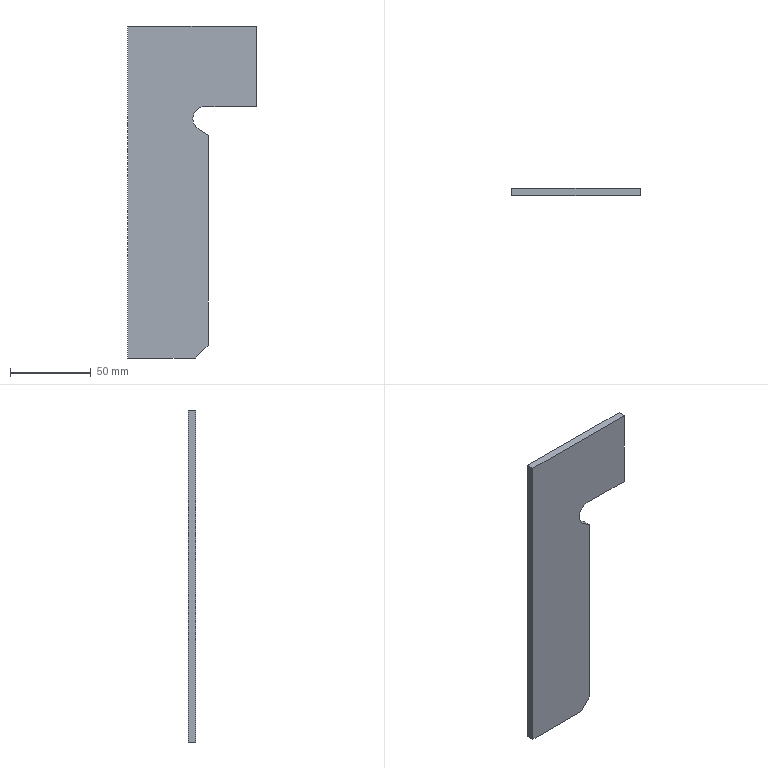Part | SolidWorks | features FlatPattern 1, SMBaseFlange 1, SheetMetal 1 | 1 solid | 11 faces | box 80 x 4.5 x 206 mm | volume 52392 mm3 | plane 10 | cylinder 1 | commonest cylinder face diameters 15 x1
STEP:
#1=CARTESIAN_POINT('',(0.,0.,0.));
#2=VERTEX_POINT('',#1);
#3=CARTESIAN_POINT('',(0.,0.,206.));
#4=VERTEX_POINT('',#3);
#5=CARTESIAN_POINT('',(0.,0.,0.));
#6=DIRECTION('',(0.,0.,1.));
#7=VECTOR('',#6,1000.);
#8=LINE('',#5,#7);
#9=EDGE_CURVE('',#2,#4,#8,.T.);
#10=ORIENTED_EDGE('',*,*,#9,.F.);
#11=CARTESIAN_POINT('',(0.,-4.5,0.));
#12=VERTEX_POINT('',#11);
#13=CARTESIAN_POINT('',(0.,-4.5,0.));
#14=DIRECTION('',(0.,1.,0.));
#15=VECTOR('',#14,1000.);
#16=LINE('',#13,#15);
#17=EDGE_CURVE('',#12,#2,#16,.T.);
#18=ORIENTED_EDGE('',*,*,#17,.F.);
#19=CARTESIAN_POINT('',(0.,-4.5,206.));
#20=VERTEX_POINT('',#19);
#21=CARTESIAN_POINT('',(0.,-4.5,0.));
#22=DIRECTION('',(0.,0.,1.));
#23=VECTOR('',#22,1000.);
#24=LINE('',#21,#23);
#25=EDGE_CURVE('',#12,#20,#24,.T.);
#26=ORIENTED_EDGE('',*,*,#25,.T.);
#27=CARTESIAN_POINT('',(0.,-4.5,206.));
#28=DIRECTION('',(0.,1.,0.));
#29=VECTOR('',#28,1000.);
#30=LINE('',#27,#29);
#31=EDGE_CURVE('',#20,#4,#30,.T.);
#32=ORIENTED_EDGE('',*,*,#31,.T.);
#33=EDGE_LOOP('',(#10,#18,#26,#32));
#34=FACE_OUTER_BOUND('',#33,.T.);
#35=CARTESIAN_POINT('',(0.,-4.5,0.));
#36=DIRECTION('',(-1.,0.,0.));
#37=DIRECTION('',(0.,0.,1.));
#38=AXIS2_PLACEMENT_3D('',#35,#36,#37);
#39=PLANE('',#38);
#40=ADVANCED_FACE('',(#34),#39,.T.);
#41=CARTESIAN_POINT('',(42.,0.,0.));
#42=VERTEX_POINT('',#41);
#43=CARTESIAN_POINT('',(0.,0.,0.));
#44=DIRECTION('',(-1.,0.,0.));
#45=VECTOR('',#44,1000.);
#46=LINE('',#43,#45);
#47=EDGE_CURVE('',#42,#2,#46,.T.);
#48=ORIENTED_EDGE('',*,*,#47,.F.);
#49=CARTESIAN_POINT('',(42.,-4.5,0.));
#50=VERTEX_POINT('',#49);
#51=CARTESIAN_POINT('',(42.,-4.5,0.));
#52=DIRECTION('',(0.,1.,0.));
#53=VECTOR('',#52,1000.);
#54=LINE('',#51,#53);
#55=EDGE_CURVE('',#50,#42,#54,.T.);
#56=ORIENTED_EDGE('',*,*,#55,.F.);
#57=CARTESIAN_POINT('',(0.,-4.5,0.));
#58=DIRECTION('',(-1.,0.,0.));
#59=VECTOR('',#58,1000.);
#60=LINE('',#57,#59);
#61=EDGE_CURVE('',#50,#12,#60,.T.);
#62=ORIENTED_EDGE('',*,*,#61,.T.);
#63=ORIENTED_EDGE('',*,*,#17,.T.);
#64=EDGE_LOOP('',(#48,#56,#62,#63));
#65=FACE_OUTER_BOUND('',#64,.T.);
#66=CARTESIAN_POINT('',(0.,-4.5,0.));
#67=DIRECTION('',(0.,0.,-1.));
#68=DIRECTION('',(-1.,0.,0.));
#69=AXIS2_PLACEMENT_3D('',#66,#67,#68);
#70=PLANE('',#69);
#71=ADVANCED_FACE('',(#65),#70,.T.);
#72=CARTESIAN_POINT('',(50.,0.,8.));
#73=VERTEX_POINT('',#72);
#74=CARTESIAN_POINT('',(42.,0.,0.));
#75=DIRECTION('',(-0.7071,0.,-0.7071));
#76=VECTOR('',#75,1000.);
#77=LINE('',#74,#76);
#78=EDGE_CURVE('',#73,#42,#77,.T.);
#79=ORIENTED_EDGE('',*,*,#78,.F.);
#80=CARTESIAN_POINT('',(50.,-4.5,8.));
#81=VERTEX_POINT('',#80);
#82=CARTESIAN_POINT('',(50.,-4.5,8.));
#83=DIRECTION('',(0.,1.,0.));
#84=VECTOR('',#83,1000.);
#85=LINE('',#82,#84);
#86=EDGE_CURVE('',#81,#73,#85,.T.);
#87=ORIENTED_EDGE('',*,*,#86,.F.);
#88=CARTESIAN_POINT('',(42.,-4.5,0.));
#89=DIRECTION('',(-0.7071,0.,-0.7071));
#90=VECTOR('',#89,1000.);
#91=LINE('',#88,#90);
#92=EDGE_CURVE('',#81,#50,#91,.T.);
#93=ORIENTED_EDGE('',*,*,#92,.T.);
#94=ORIENTED_EDGE('',*,*,#55,.T.);
#95=EDGE_LOOP('',(#79,#87,#93,#94));
#96=FACE_OUTER_BOUND('',#95,.T.);
#97=CARTESIAN_POINT('',(42.,-4.5,0.));
#98=DIRECTION('',(0.7071,0.,-0.7071));
#99=DIRECTION('',(-0.7071,0.,-0.7071));
#100=AXIS2_PLACEMENT_3D('',#97,#98,#99);
#101=PLANE('',#100);
#102=ADVANCED_FACE('',(#96),#101,.T.);
#103=CARTESIAN_POINT('',(50.,0.,138.));
#104=VERTEX_POINT('',#103);
#105=CARTESIAN_POINT('',(50.,0.,8.));
#106=DIRECTION('',(0.,0.,-1.));
#107=VECTOR('',#106,1000.);
#108=LINE('',#105,#107);
#109=EDGE_CURVE('',#104,#73,#108,.T.);
#110=ORIENTED_EDGE('',*,*,#109,.F.);
#111=CARTESIAN_POINT('',(50.,-4.5,138.));
#112=VERTEX_POINT('',#111);
#113=CARTESIAN_POINT('',(50.,-4.5,138.));
#114=DIRECTION('',(0.,1.,0.));
#115=VECTOR('',#114,1000.);
#116=LINE('',#113,#115);
#117=EDGE_CURVE('',#112,#104,#116,.T.);
#118=ORIENTED_EDGE('',*,*,#117,.F.);
#119=CARTESIAN_POINT('',(50.,-4.5,8.));
#120=DIRECTION('',(0.,0.,-1.));
#121=VECTOR('',#120,1000.);
#122=LINE('',#119,#121);
#123=EDGE_CURVE('',#112,#81,#122,.T.);
#124=ORIENTED_EDGE('',*,*,#123,.T.);
#125=ORIENTED_EDGE('',*,*,#86,.T.);
#126=EDGE_LOOP('',(#110,#118,#124,#125));
#127=FACE_OUTER_BOUND('',#126,.T.);
#128=CARTESIAN_POINT('',(50.,-4.5,8.));
#129=DIRECTION('',(1.,0.,0.));
#130=DIRECTION('',(0.,0.,-1.));
#131=AXIS2_PLACEMENT_3D('',#128,#129,#130);
#132=PLANE('',#131);
#133=ADVANCED_FACE('',(#127),#132,.T.);
#134=CARTESIAN_POINT('',(43.735,0.,142.331));
#135=VERTEX_POINT('',#134);
#136=CARTESIAN_POINT('',(50.,0.,138.));
#137=DIRECTION('',(0.8226,0.,-0.5686));
#138=VECTOR('',#137,1000.);
#139=LINE('',#136,#138);
#140=EDGE_CURVE('',#135,#104,#139,.T.);
#141=ORIENTED_EDGE('',*,*,#140,.F.);
#142=CARTESIAN_POINT('',(43.735,-4.5,142.331));
#143=VERTEX_POINT('',#142);
#144=CARTESIAN_POINT('',(43.735,-4.5,142.331));
#145=DIRECTION('',(0.,1.,0.));
#146=VECTOR('',#145,1000.);
#147=LINE('',#144,#146);
#148=EDGE_CURVE('',#143,#135,#147,.T.);
#149=ORIENTED_EDGE('',*,*,#148,.F.);
#150=CARTESIAN_POINT('',(50.,-4.5,138.));
#151=DIRECTION('',(0.8226,0.,-0.5686));
#152=VECTOR('',#151,1000.);
#153=LINE('',#150,#152);
#154=EDGE_CURVE('',#143,#112,#153,.T.);
#155=ORIENTED_EDGE('',*,*,#154,.T.);
#156=ORIENTED_EDGE('',*,*,#117,.T.);
#157=EDGE_LOOP('',(#141,#149,#155,#156));
#158=FACE_OUTER_BOUND('',#157,.T.);
#159=CARTESIAN_POINT('',(50.,-4.5,138.));
#160=DIRECTION('',(0.5686,0.,0.8226));
#161=DIRECTION('',(0.8226,0.,-0.5686));
#162=AXIS2_PLACEMENT_3D('',#159,#160,#161);
#163=PLANE('',#162);
#164=ADVANCED_FACE('',(#158),#163,.T.);
#165=CARTESIAN_POINT('',(48.,0.,156.));
#166=VERTEX_POINT('',#165);
#167=CARTESIAN_POINT('',(48.,0.,148.5));
#168=DIRECTION('',(0.,-1.,0.));
#169=DIRECTION('',(0.,0.,1.));
#170=AXIS2_PLACEMENT_3D('',#167,#168,#169);
#171=CIRCLE('',#170,7.5);
#172=EDGE_CURVE('',#166,#135,#171,.T.);
#173=ORIENTED_EDGE('',*,*,#172,.F.);
#174=CARTESIAN_POINT('',(48.,-4.5,156.));
#175=VERTEX_POINT('',#174);
#176=CARTESIAN_POINT('',(48.,-4.5,156.));
#177=DIRECTION('',(0.,1.,0.));
#178=VECTOR('',#177,1000.);
#179=LINE('',#176,#178);
#180=EDGE_CURVE('',#175,#166,#179,.T.);
#181=ORIENTED_EDGE('',*,*,#180,.F.);
#182=CARTESIAN_POINT('',(48.,-4.5,148.5));
#183=DIRECTION('',(0.,-1.,0.));
#184=DIRECTION('',(0.,0.,1.));
#185=AXIS2_PLACEMENT_3D('',#182,#183,#184);
#186=CIRCLE('',#185,7.5);
#187=EDGE_CURVE('',#175,#143,#186,.T.);
#188=ORIENTED_EDGE('',*,*,#187,.T.);
#189=ORIENTED_EDGE('',*,*,#148,.T.);
#190=EDGE_LOOP('',(#173,#181,#188,#189));
#191=FACE_OUTER_BOUND('',#190,.T.);
#192=CARTESIAN_POINT('',(48.,-4.5,148.5));
#193=DIRECTION('',(0.,1.,0.));
#194=DIRECTION('',(0.,0.,1.));
#195=AXIS2_PLACEMENT_3D('',#192,#193,#194);
#196=CYLINDRICAL_SURFACE('',#195,7.5);
#197=ADVANCED_FACE('',(#191),#196,.F.);
#198=CARTESIAN_POINT('',(80.,0.,156.));
#199=VERTEX_POINT('',#198);
#200=CARTESIAN_POINT('',(48.,0.,156.));
#201=DIRECTION('',(-1.,0.,0.));
#202=VECTOR('',#201,1000.);
#203=LINE('',#200,#202);
#204=EDGE_CURVE('',#199,#166,#203,.T.);
#205=ORIENTED_EDGE('',*,*,#204,.F.);
#206=CARTESIAN_POINT('',(80.,-4.5,156.));
#207=VERTEX_POINT('',#206);
#208=CARTESIAN_POINT('',(80.,-4.5,156.));
#209=DIRECTION('',(0.,1.,0.));
#210=VECTOR('',#209,1000.);
#211=LINE('',#208,#210);
#212=EDGE_CURVE('',#207,#199,#211,.T.);
#213=ORIENTED_EDGE('',*,*,#212,.F.);
#214=CARTESIAN_POINT('',(48.,-4.5,156.));
#215=DIRECTION('',(-1.,0.,0.));
#216=VECTOR('',#215,1000.);
#217=LINE('',#214,#216);
#218=EDGE_CURVE('',#207,#175,#217,.T.);
#219=ORIENTED_EDGE('',*,*,#218,.T.);
#220=ORIENTED_EDGE('',*,*,#180,.T.);
#221=EDGE_LOOP('',(#205,#213,#219,#220));
#222=FACE_OUTER_BOUND('',#221,.T.);
#223=CARTESIAN_POINT('',(48.,-4.5,156.));
#224=DIRECTION('',(0.,0.,-1.));
#225=DIRECTION('',(-1.,0.,0.));
#226=AXIS2_PLACEMENT_3D('',#223,#224,#225);
#227=PLANE('',#226);
#228=ADVANCED_FACE('',(#222),#227,.T.);
#229=CARTESIAN_POINT('',(80.,0.,206.));
#230=VERTEX_POINT('',#229);
#231=CARTESIAN_POINT('',(80.,0.,156.));
#232=DIRECTION('',(0.,0.,-1.));
#233=VECTOR('',#232,1000.);
#234=LINE('',#231,#233);
#235=EDGE_CURVE('',#230,#199,#234,.T.);
#236=ORIENTED_EDGE('',*,*,#235,.F.);
#237=CARTESIAN_POINT('',(80.,-4.5,206.));
#238=VERTEX_POINT('',#237);
#239=CARTESIAN_POINT('',(80.,-4.5,206.));
#240=DIRECTION('',(0.,1.,0.));
#241=VECTOR('',#240,1000.);
#242=LINE('',#239,#241);
#243=EDGE_CURVE('',#238,#230,#242,.T.);
#244=ORIENTED_EDGE('',*,*,#243,.F.);
#245=CARTESIAN_POINT('',(80.,-4.5,156.));
#246=DIRECTION('',(0.,0.,-1.));
#247=VECTOR('',#246,1000.);
#248=LINE('',#245,#247);
#249=EDGE_CURVE('',#238,#207,#248,.T.);
#250=ORIENTED_EDGE('',*,*,#249,.T.);
#251=ORIENTED_EDGE('',*,*,#212,.T.);
#252=EDGE_LOOP('',(#236,#244,#250,#251));
#253=FACE_OUTER_BOUND('',#252,.T.);
#254=CARTESIAN_POINT('',(80.,-4.5,156.));
#255=DIRECTION('',(1.,0.,0.));
#256=DIRECTION('',(0.,0.,-1.));
#257=AXIS2_PLACEMENT_3D('',#254,#255,#256);
#258=PLANE('',#257);
#259=ADVANCED_FACE('',(#253),#258,.T.);
#260=CARTESIAN_POINT('',(0.,0.,206.));
#261=DIRECTION('',(1.,0.,0.));
#262=VECTOR('',#261,1000.);
#263=LINE('',#260,#262);
#264=EDGE_CURVE('',#4,#230,#263,.T.);
#265=ORIENTED_EDGE('',*,*,#264,.F.);
#266=ORIENTED_EDGE('',*,*,#31,.F.);
#267=CARTESIAN_POINT('',(0.,-4.5,206.));
#268=DIRECTION('',(1.,0.,0.));
#269=VECTOR('',#268,1000.);
#270=LINE('',#267,#269);
#271=EDGE_CURVE('',#20,#238,#270,.T.);
#272=ORIENTED_EDGE('',*,*,#271,.T.);
#273=ORIENTED_EDGE('',*,*,#243,.T.);
#274=EDGE_LOOP('',(#265,#266,#272,#273));
#275=FACE_OUTER_BOUND('',#274,.T.);
#276=CARTESIAN_POINT('',(0.,-4.5,206.));
#277=DIRECTION('',(0.,0.,1.));
#278=DIRECTION('',(1.,0.,0.));
#279=AXIS2_PLACEMENT_3D('',#276,#277,#278);
#280=PLANE('',#279);
#281=ADVANCED_FACE('',(#275),#280,.T.);
#282=ORIENTED_EDGE('',*,*,#25,.F.);
#283=ORIENTED_EDGE('',*,*,#61,.F.);
#284=ORIENTED_EDGE('',*,*,#92,.F.);
#285=ORIENTED_EDGE('',*,*,#123,.F.);
#286=ORIENTED_EDGE('',*,*,#154,.F.);
#287=ORIENTED_EDGE('',*,*,#187,.F.);
#288=ORIENTED_EDGE('',*,*,#218,.F.);
#289=ORIENTED_EDGE('',*,*,#249,.F.);
#290=ORIENTED_EDGE('',*,*,#271,.F.);
#291=EDGE_LOOP('',(#282,#283,#284,#285,#286,#287,#288,#289,#290));
#292=FACE_OUTER_BOUND('',#291,.T.);
#293=CARTESIAN_POINT('',(48.,-4.5,148.5));
#294=DIRECTION('',(0.,1.,0.));
#295=DIRECTION('',(0.,0.,1.));
#296=AXIS2_PLACEMENT_3D('',#293,#294,#295);
#297=PLANE('',#296);
#298=ADVANCED_FACE('',(#292),#297,.F.);
#299=ORIENTED_EDGE('',*,*,#9,.T.);
#300=ORIENTED_EDGE('',*,*,#264,.T.);
#301=ORIENTED_EDGE('',*,*,#235,.T.);
#302=ORIENTED_EDGE('',*,*,#204,.T.);
#303=ORIENTED_EDGE('',*,*,#172,.T.);
#304=ORIENTED_EDGE('',*,*,#140,.T.);
#305=ORIENTED_EDGE('',*,*,#109,.T.);
#306=ORIENTED_EDGE('',*,*,#78,.T.);
#307=ORIENTED_EDGE('',*,*,#47,.T.);
#308=EDGE_LOOP('',(#299,#300,#301,#302,#303,#304,#305,#306,#307));
#309=FACE_OUTER_BOUND('',#308,.T.);
#310=CARTESIAN_POINT('',(48.,0.,148.5));
#311=DIRECTION('',(0.,1.,0.));
#312=DIRECTION('',(0.,0.,1.));
#313=AXIS2_PLACEMENT_3D('',#310,#311,#312);
#314=PLANE('',#313);
#315=ADVANCED_FACE('',(#309),#314,.T.);
#316=CLOSED_SHELL('',(#40,#71,#102,#133,#164,#197,#228,#259,#281,#298,#315));
#317=MANIFOLD_SOLID_BREP('',#316);
#318=CARTESIAN_POINT('',(0.,0.,0.));
#319=DIRECTION('',(0.,0.,1.));
#320=DIRECTION('',(1.,0.,0.));
#321=AXIS2_PLACEMENT_3D('',#318,#319,#320);
#322=(LENGTH_UNIT()NAMED_UNIT(*)SI_UNIT(.MILLI.,.METRE.));
#323=UNCERTAINTY_MEASURE_WITH_UNIT(LENGTH_MEASURE(0.00001),#322,'','');
#324=(NAMED_UNIT(*)PLANE_ANGLE_UNIT()SI_UNIT($,.RADIAN.));
#325=(NAMED_UNIT(*)SI_UNIT($,.STERADIAN.)SOLID_ANGLE_UNIT());
#326=(GEOMETRIC_REPRESENTATION_CONTEXT(3)GLOBAL_UNCERTAINTY_ASSIGNED_CONTEXT((#323))GLOBAL_UNIT_ASSIGNED_CONTEXT((#322,#324,#325))REPRESENTATION_CONTEXT('',''));
#327=ADVANCED_BREP_SHAPE_REPRESENTATION('',(#317,#321),#326);